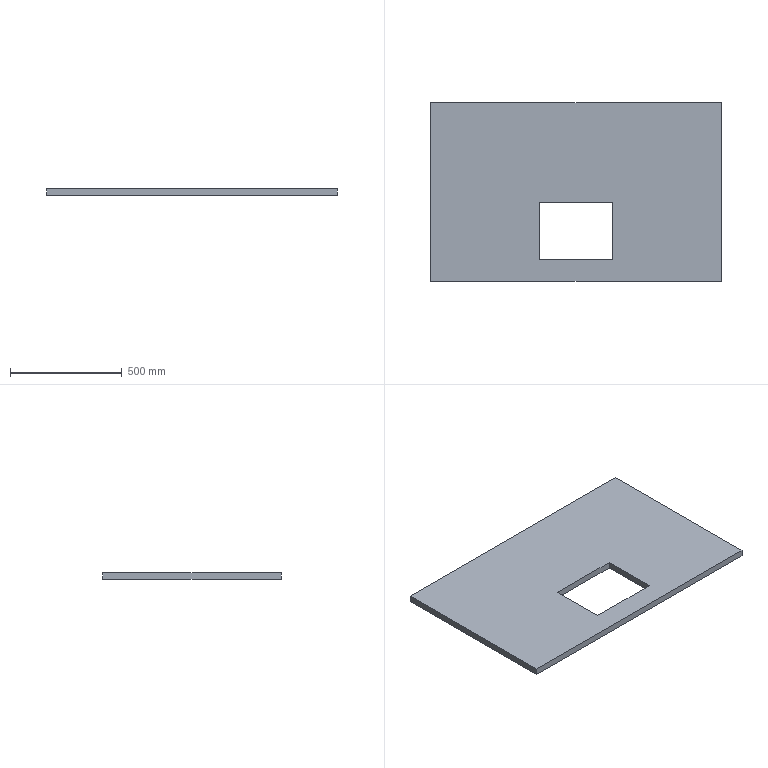Part | STEP file | Tube necking machine_id670_x_t | 1 solid | 10 faces | box 1300 x 800 x 30 mm | volume 28708260 mm3 | plane 10
STEP:
#1=CARTESIAN_POINT('',(0.,0.,0.));
#2=DIRECTION('',(0.,0.,1.));
#3=DIRECTION('',(1.,0.,0.));
#4=AXIS2_PLACEMENT_3D('',#1,#2,#3);
#5=CARTESIAN_POINT('',(-650.,400.,-30.));
#6=VERTEX_POINT('',#5);
#7=CARTESIAN_POINT('',(-650.,-400.,-30.));
#8=VERTEX_POINT('',#7);
#9=CARTESIAN_POINT('',(-650.,400.,-30.));
#10=DIRECTION('',(0.,-1.,0.));
#11=VECTOR('',#10,1.);
#12=LINE('',#9,#11);
#13=CARTESIAN_POINT('',(0.,0.,-30.));
#14=DIRECTION('',(0.,0.,1.));
#15=DIRECTION('',(1.,0.,0.));
#16=AXIS2_PLACEMENT_3D('',#13,#14,#15);
#17=PLANE('',#16);
#18=CARTESIAN_POINT('',(-650.,400.));
#19=DIRECTION('',(0.,-1.));
#20=VECTOR('',#19,1.);
#21=LINE('',#18,#20);
#22=(GEOMETRIC_REPRESENTATION_CONTEXT(2)PARAMETRIC_REPRESENTATION_CONTEXT()REPRESENTATION_CONTEXT('',''));
#23=DEFINITIONAL_REPRESENTATION('',(#21),#22);
#24=PCURVE('',#17,#23);
#25=CARTESIAN_POINT('',(-650.,400.,-30.));
#26=DIRECTION('',(-1.,0.,0.));
#27=DIRECTION('',(0.,0.,1.));
#28=AXIS2_PLACEMENT_3D('',#25,#26,#27);
#29=PLANE('',#28);
#30=CARTESIAN_POINT('',(0.,0.));
#31=DIRECTION('',(0.,-1.));
#32=VECTOR('',#31,1.);
#33=LINE('',#30,#32);
#34=(GEOMETRIC_REPRESENTATION_CONTEXT(2)PARAMETRIC_REPRESENTATION_CONTEXT()REPRESENTATION_CONTEXT('',''));
#35=DEFINITIONAL_REPRESENTATION('',(#33),#34);
#36=PCURVE('',#29,#35);
#37=SURFACE_CURVE('',#12,(#24,#36),.PCURVE_S1.);
#38=EDGE_CURVE('',#6,#8,#37,.T.);
#39=ORIENTED_EDGE('',*,*,#38,.F.);
#40=CARTESIAN_POINT('',(650.,400.,-30.));
#41=VERTEX_POINT('',#40);
#42=CARTESIAN_POINT('',(650.,400.,-30.));
#43=DIRECTION('',(-1.,0.,0.));
#44=VECTOR('',#43,1.);
#45=LINE('',#42,#44);
#46=CARTESIAN_POINT('',(650.,400.));
#47=DIRECTION('',(-1.,0.));
#48=VECTOR('',#47,1.);
#49=LINE('',#46,#48);
#50=(GEOMETRIC_REPRESENTATION_CONTEXT(2)PARAMETRIC_REPRESENTATION_CONTEXT()REPRESENTATION_CONTEXT('',''));
#51=DEFINITIONAL_REPRESENTATION('',(#49),#50);
#52=PCURVE('',#17,#51);
#53=CARTESIAN_POINT('',(650.,400.,-30.));
#54=DIRECTION('',(0.,1.,0.));
#55=DIRECTION('',(0.,0.,1.));
#56=AXIS2_PLACEMENT_3D('',#53,#54,#55);
#57=PLANE('',#56);
#58=CARTESIAN_POINT('',(0.,0.));
#59=DIRECTION('',(0.,-1.));
#60=VECTOR('',#59,1.);
#61=LINE('',#58,#60);
#62=(GEOMETRIC_REPRESENTATION_CONTEXT(2)PARAMETRIC_REPRESENTATION_CONTEXT()REPRESENTATION_CONTEXT('',''));
#63=DEFINITIONAL_REPRESENTATION('',(#61),#62);
#64=PCURVE('',#57,#63);
#65=SURFACE_CURVE('',#45,(#52,#64),.PCURVE_S1.);
#66=EDGE_CURVE('',#41,#6,#65,.T.);
#67=ORIENTED_EDGE('',*,*,#66,.F.);
#68=CARTESIAN_POINT('',(650.,-400.,-30.));
#69=VERTEX_POINT('',#68);
#70=CARTESIAN_POINT('',(650.,-400.,-30.));
#71=DIRECTION('',(0.,1.,0.));
#72=VECTOR('',#71,1.);
#73=LINE('',#70,#72);
#74=CARTESIAN_POINT('',(650.,-400.));
#75=DIRECTION('',(0.,1.));
#76=VECTOR('',#75,1.);
#77=LINE('',#74,#76);
#78=(GEOMETRIC_REPRESENTATION_CONTEXT(2)PARAMETRIC_REPRESENTATION_CONTEXT()REPRESENTATION_CONTEXT('',''));
#79=DEFINITIONAL_REPRESENTATION('',(#77),#78);
#80=PCURVE('',#17,#79);
#81=CARTESIAN_POINT('',(650.,-400.,-30.));
#82=DIRECTION('',(1.,0.,0.));
#83=DIRECTION('',(0.,0.,-1.));
#84=AXIS2_PLACEMENT_3D('',#81,#82,#83);
#85=PLANE('',#84);
#86=CARTESIAN_POINT('',(0.,0.));
#87=DIRECTION('',(0.,1.));
#88=VECTOR('',#87,1.);
#89=LINE('',#86,#88);
#90=(GEOMETRIC_REPRESENTATION_CONTEXT(2)PARAMETRIC_REPRESENTATION_CONTEXT()REPRESENTATION_CONTEXT('',''));
#91=DEFINITIONAL_REPRESENTATION('',(#89),#90);
#92=PCURVE('',#85,#91);
#93=SURFACE_CURVE('',#73,(#80,#92),.PCURVE_S1.);
#94=EDGE_CURVE('',#69,#41,#93,.T.);
#95=ORIENTED_EDGE('',*,*,#94,.F.);
#96=CARTESIAN_POINT('',(-650.,-400.,-30.));
#97=DIRECTION('',(1.,0.,0.));
#98=VECTOR('',#97,1.);
#99=LINE('',#96,#98);
#100=CARTESIAN_POINT('',(-650.,-400.));
#101=DIRECTION('',(1.,0.));
#102=VECTOR('',#101,1.);
#103=LINE('',#100,#102);
#104=(GEOMETRIC_REPRESENTATION_CONTEXT(2)PARAMETRIC_REPRESENTATION_CONTEXT()REPRESENTATION_CONTEXT('',''));
#105=DEFINITIONAL_REPRESENTATION('',(#103),#104);
#106=PCURVE('',#17,#105);
#107=CARTESIAN_POINT('',(-650.,-400.,-30.));
#108=DIRECTION('',(0.,-1.,0.));
#109=DIRECTION('',(0.,0.,-1.));
#110=AXIS2_PLACEMENT_3D('',#107,#108,#109);
#111=PLANE('',#110);
#112=CARTESIAN_POINT('',(0.,0.));
#113=DIRECTION('',(0.,1.));
#114=VECTOR('',#113,1.);
#115=LINE('',#112,#114);
#116=(GEOMETRIC_REPRESENTATION_CONTEXT(2)PARAMETRIC_REPRESENTATION_CONTEXT()REPRESENTATION_CONTEXT('',''));
#117=DEFINITIONAL_REPRESENTATION('',(#115),#116);
#118=PCURVE('',#111,#117);
#119=SURFACE_CURVE('',#99,(#106,#118),.PCURVE_S1.);
#120=EDGE_CURVE('',#8,#69,#119,.T.);
#121=ORIENTED_EDGE('',*,*,#120,.F.);
#122=EDGE_LOOP('',(#39,#67,#95,#121));
#123=FACE_BOUND('',#122,.T.);
#124=CARTESIAN_POINT('',(-163.5,-46.,-30.));
#125=VERTEX_POINT('',#124);
#126=CARTESIAN_POINT('',(-163.5,-300.,-30.));
#127=VERTEX_POINT('',#126);
#128=CARTESIAN_POINT('',(-163.5,0.,-30.));
#129=DIRECTION('',(0.,-1.,0.));
#130=VECTOR('',#129,1.);
#131=LINE('',#128,#130);
#132=CARTESIAN_POINT('',(-163.5,0.));
#133=DIRECTION('',(0.,-1.));
#134=VECTOR('',#133,1.);
#135=LINE('',#132,#134);
#136=(GEOMETRIC_REPRESENTATION_CONTEXT(2)PARAMETRIC_REPRESENTATION_CONTEXT()REPRESENTATION_CONTEXT('',''));
#137=DEFINITIONAL_REPRESENTATION('',(#135),#136);
#138=PCURVE('',#17,#137);
#139=CARTESIAN_POINT('',(-163.5,-46.,30.));
#140=DIRECTION('',(1.,0.,0.));
#141=DIRECTION('',(0.,0.,-1.));
#142=AXIS2_PLACEMENT_3D('',#139,#140,#141);
#143=PLANE('',#142);
#144=CARTESIAN_POINT('',(60.,46.));
#145=DIRECTION('',(0.,-1.));
#146=VECTOR('',#145,1.);
#147=LINE('',#144,#146);
#148=(GEOMETRIC_REPRESENTATION_CONTEXT(2)PARAMETRIC_REPRESENTATION_CONTEXT()REPRESENTATION_CONTEXT('',''));
#149=DEFINITIONAL_REPRESENTATION('',(#147),#148);
#150=PCURVE('',#143,#149);
#151=SURFACE_CURVE('',#131,(#138,#150),.PCURVE_S1.);
#152=EDGE_CURVE('',#125,#127,#151,.T.);
#153=ORIENTED_EDGE('',*,*,#152,.T.);
#154=CARTESIAN_POINT('',(163.5,-300.,-30.));
#155=VERTEX_POINT('',#154);
#156=CARTESIAN_POINT('',(0.,-300.,-30.));
#157=DIRECTION('',(1.,0.,0.));
#158=VECTOR('',#157,1.);
#159=LINE('',#156,#158);
#160=CARTESIAN_POINT('',(0.,-300.));
#161=DIRECTION('',(1.,0.));
#162=VECTOR('',#161,1.);
#163=LINE('',#160,#162);
#164=(GEOMETRIC_REPRESENTATION_CONTEXT(2)PARAMETRIC_REPRESENTATION_CONTEXT()REPRESENTATION_CONTEXT('',''));
#165=DEFINITIONAL_REPRESENTATION('',(#163),#164);
#166=PCURVE('',#17,#165);
#167=CARTESIAN_POINT('',(-163.5,-300.,30.));
#168=DIRECTION('',(0.,1.,0.));
#169=DIRECTION('',(0.,0.,1.));
#170=AXIS2_PLACEMENT_3D('',#167,#168,#169);
#171=PLANE('',#170);
#172=CARTESIAN_POINT('',(-60.,163.5));
#173=DIRECTION('',(0.,1.));
#174=VECTOR('',#173,1.);
#175=LINE('',#172,#174);
#176=(GEOMETRIC_REPRESENTATION_CONTEXT(2)PARAMETRIC_REPRESENTATION_CONTEXT()REPRESENTATION_CONTEXT('',''));
#177=DEFINITIONAL_REPRESENTATION('',(#175),#176);
#178=PCURVE('',#171,#177);
#179=SURFACE_CURVE('',#159,(#166,#178),.PCURVE_S1.);
#180=EDGE_CURVE('',#127,#155,#179,.T.);
#181=ORIENTED_EDGE('',*,*,#180,.T.);
#182=CARTESIAN_POINT('',(163.5,-46.,-30.));
#183=VERTEX_POINT('',#182);
#184=CARTESIAN_POINT('',(163.5,0.,-30.));
#185=DIRECTION('',(0.,1.,0.));
#186=VECTOR('',#185,1.);
#187=LINE('',#184,#186);
#188=CARTESIAN_POINT('',(163.5,0.));
#189=DIRECTION('',(0.,1.));
#190=VECTOR('',#189,1.);
#191=LINE('',#188,#190);
#192=(GEOMETRIC_REPRESENTATION_CONTEXT(2)PARAMETRIC_REPRESENTATION_CONTEXT()REPRESENTATION_CONTEXT('',''));
#193=DEFINITIONAL_REPRESENTATION('',(#191),#192);
#194=PCURVE('',#17,#193);
#195=CARTESIAN_POINT('',(163.5,-300.,30.));
#196=DIRECTION('',(-1.,0.,0.));
#197=DIRECTION('',(0.,-1.,0.));
#198=AXIS2_PLACEMENT_3D('',#195,#196,#197);
#199=PLANE('',#198);
#200=CARTESIAN_POINT('',(-300.,-60.));
#201=DIRECTION('',(-1.,0.));
#202=VECTOR('',#201,1.);
#203=LINE('',#200,#202);
#204=(GEOMETRIC_REPRESENTATION_CONTEXT(2)PARAMETRIC_REPRESENTATION_CONTEXT()REPRESENTATION_CONTEXT('',''));
#205=DEFINITIONAL_REPRESENTATION('',(#203),#204);
#206=PCURVE('',#199,#205);
#207=SURFACE_CURVE('',#187,(#194,#206),.PCURVE_S1.);
#208=EDGE_CURVE('',#155,#183,#207,.T.);
#209=ORIENTED_EDGE('',*,*,#208,.T.);
#210=CARTESIAN_POINT('',(0.,-46.,-30.));
#211=DIRECTION('',(-1.,0.,0.));
#212=VECTOR('',#211,1.);
#213=LINE('',#210,#212);
#214=CARTESIAN_POINT('',(0.,-46.));
#215=DIRECTION('',(-1.,0.));
#216=VECTOR('',#215,1.);
#217=LINE('',#214,#216);
#218=(GEOMETRIC_REPRESENTATION_CONTEXT(2)PARAMETRIC_REPRESENTATION_CONTEXT()REPRESENTATION_CONTEXT('',''));
#219=DEFINITIONAL_REPRESENTATION('',(#217),#218);
#220=PCURVE('',#17,#219);
#221=CARTESIAN_POINT('',(163.5,-46.,30.));
#222=DIRECTION('',(0.,-1.,0.));
#223=DIRECTION('',(0.,0.,-1.));
#224=AXIS2_PLACEMENT_3D('',#221,#222,#223);
#225=PLANE('',#224);
#226=CARTESIAN_POINT('',(60.,-163.5));
#227=DIRECTION('',(0.,-1.));
#228=VECTOR('',#227,1.);
#229=LINE('',#226,#228);
#230=(GEOMETRIC_REPRESENTATION_CONTEXT(2)PARAMETRIC_REPRESENTATION_CONTEXT()REPRESENTATION_CONTEXT('',''));
#231=DEFINITIONAL_REPRESENTATION('',(#229),#230);
#232=PCURVE('',#225,#231);
#233=SURFACE_CURVE('',#213,(#220,#232),.PCURVE_S1.);
#234=EDGE_CURVE('',#183,#125,#233,.T.);
#235=ORIENTED_EDGE('',*,*,#234,.T.);
#236=EDGE_LOOP('',(#153,#181,#209,#235));
#237=FACE_BOUND('',#236,.T.);
#238=ADVANCED_FACE('',(#123,#237),#17,.F.);
#239=CARTESIAN_POINT('',(-650.,400.,0.));
#240=VERTEX_POINT('',#239);
#241=CARTESIAN_POINT('',(-650.,-400.,0.));
#242=VERTEX_POINT('',#241);
#243=CARTESIAN_POINT('',(-650.,400.,0.));
#244=DIRECTION('',(0.,-1.,0.));
#245=VECTOR('',#244,1.);
#246=LINE('',#243,#245);
#247=CARTESIAN_POINT('',(0.,0.,0.));
#248=DIRECTION('',(0.,0.,1.));
#249=DIRECTION('',(1.,0.,0.));
#250=AXIS2_PLACEMENT_3D('',#247,#248,#249);
#251=PLANE('',#250);
#252=CARTESIAN_POINT('',(-650.,400.));
#253=DIRECTION('',(0.,-1.));
#254=VECTOR('',#253,1.);
#255=LINE('',#252,#254);
#256=(GEOMETRIC_REPRESENTATION_CONTEXT(2)PARAMETRIC_REPRESENTATION_CONTEXT()REPRESENTATION_CONTEXT('',''));
#257=DEFINITIONAL_REPRESENTATION('',(#255),#256);
#258=PCURVE('',#251,#257);
#259=CARTESIAN_POINT('',(30.,0.));
#260=DIRECTION('',(0.,-1.));
#261=VECTOR('',#260,1.);
#262=LINE('',#259,#261);
#263=(GEOMETRIC_REPRESENTATION_CONTEXT(2)PARAMETRIC_REPRESENTATION_CONTEXT()REPRESENTATION_CONTEXT('',''));
#264=DEFINITIONAL_REPRESENTATION('',(#262),#263);
#265=PCURVE('',#29,#264);
#266=SURFACE_CURVE('',#246,(#258,#265),.PCURVE_S1.);
#267=EDGE_CURVE('',#240,#242,#266,.T.);
#268=ORIENTED_EDGE('',*,*,#267,.T.);
#269=CARTESIAN_POINT('',(650.,-400.,0.));
#270=VERTEX_POINT('',#269);
#271=CARTESIAN_POINT('',(-650.,-400.,0.));
#272=DIRECTION('',(1.,0.,0.));
#273=VECTOR('',#272,1.);
#274=LINE('',#271,#273);
#275=CARTESIAN_POINT('',(-650.,-400.));
#276=DIRECTION('',(1.,0.));
#277=VECTOR('',#276,1.);
#278=LINE('',#275,#277);
#279=(GEOMETRIC_REPRESENTATION_CONTEXT(2)PARAMETRIC_REPRESENTATION_CONTEXT()REPRESENTATION_CONTEXT('',''));
#280=DEFINITIONAL_REPRESENTATION('',(#278),#279);
#281=PCURVE('',#251,#280);
#282=CARTESIAN_POINT('',(-30.,0.));
#283=DIRECTION('',(0.,1.));
#284=VECTOR('',#283,1.);
#285=LINE('',#282,#284);
#286=(GEOMETRIC_REPRESENTATION_CONTEXT(2)PARAMETRIC_REPRESENTATION_CONTEXT()REPRESENTATION_CONTEXT('',''));
#287=DEFINITIONAL_REPRESENTATION('',(#285),#286);
#288=PCURVE('',#111,#287);
#289=SURFACE_CURVE('',#274,(#281,#288),.PCURVE_S1.);
#290=EDGE_CURVE('',#242,#270,#289,.T.);
#291=ORIENTED_EDGE('',*,*,#290,.T.);
#292=CARTESIAN_POINT('',(650.,400.,0.));
#293=VERTEX_POINT('',#292);
#294=CARTESIAN_POINT('',(650.,-400.,0.));
#295=DIRECTION('',(0.,1.,0.));
#296=VECTOR('',#295,1.);
#297=LINE('',#294,#296);
#298=CARTESIAN_POINT('',(650.,-400.));
#299=DIRECTION('',(0.,1.));
#300=VECTOR('',#299,1.);
#301=LINE('',#298,#300);
#302=(GEOMETRIC_REPRESENTATION_CONTEXT(2)PARAMETRIC_REPRESENTATION_CONTEXT()REPRESENTATION_CONTEXT('',''));
#303=DEFINITIONAL_REPRESENTATION('',(#301),#302);
#304=PCURVE('',#251,#303);
#305=CARTESIAN_POINT('',(-30.,0.));
#306=DIRECTION('',(0.,1.));
#307=VECTOR('',#306,1.);
#308=LINE('',#305,#307);
#309=(GEOMETRIC_REPRESENTATION_CONTEXT(2)PARAMETRIC_REPRESENTATION_CONTEXT()REPRESENTATION_CONTEXT('',''));
#310=DEFINITIONAL_REPRESENTATION('',(#308),#309);
#311=PCURVE('',#85,#310);
#312=SURFACE_CURVE('',#297,(#304,#311),.PCURVE_S1.);
#313=EDGE_CURVE('',#270,#293,#312,.T.);
#314=ORIENTED_EDGE('',*,*,#313,.T.);
#315=CARTESIAN_POINT('',(650.,400.,0.));
#316=DIRECTION('',(-1.,0.,0.));
#317=VECTOR('',#316,1.);
#318=LINE('',#315,#317);
#319=CARTESIAN_POINT('',(650.,400.));
#320=DIRECTION('',(-1.,0.));
#321=VECTOR('',#320,1.);
#322=LINE('',#319,#321);
#323=(GEOMETRIC_REPRESENTATION_CONTEXT(2)PARAMETRIC_REPRESENTATION_CONTEXT()REPRESENTATION_CONTEXT('',''));
#324=DEFINITIONAL_REPRESENTATION('',(#322),#323);
#325=PCURVE('',#251,#324);
#326=CARTESIAN_POINT('',(30.,0.));
#327=DIRECTION('',(0.,-1.));
#328=VECTOR('',#327,1.);
#329=LINE('',#326,#328);
#330=(GEOMETRIC_REPRESENTATION_CONTEXT(2)PARAMETRIC_REPRESENTATION_CONTEXT()REPRESENTATION_CONTEXT('',''));
#331=DEFINITIONAL_REPRESENTATION('',(#329),#330);
#332=PCURVE('',#57,#331);
#333=SURFACE_CURVE('',#318,(#325,#332),.PCURVE_S1.);
#334=EDGE_CURVE('',#293,#240,#333,.T.);
#335=ORIENTED_EDGE('',*,*,#334,.T.);
#336=EDGE_LOOP('',(#268,#291,#314,#335));
#337=FACE_BOUND('',#336,.T.);
#338=CARTESIAN_POINT('',(-163.5,-300.,0.));
#339=VERTEX_POINT('',#338);
#340=CARTESIAN_POINT('',(163.5,-300.,0.));
#341=VERTEX_POINT('',#340);
#342=CARTESIAN_POINT('',(0.,-300.,0.));
#343=DIRECTION('',(1.,0.,0.));
#344=VECTOR('',#343,1.);
#345=LINE('',#342,#344);
#346=CARTESIAN_POINT('',(0.,-300.));
#347=DIRECTION('',(1.,0.));
#348=VECTOR('',#347,1.);
#349=LINE('',#346,#348);
#350=(GEOMETRIC_REPRESENTATION_CONTEXT(2)PARAMETRIC_REPRESENTATION_CONTEXT()REPRESENTATION_CONTEXT('',''));
#351=DEFINITIONAL_REPRESENTATION('',(#349),#350);
#352=PCURVE('',#251,#351);
#353=CARTESIAN_POINT('',(-30.,163.5));
#354=DIRECTION('',(0.,1.));
#355=VECTOR('',#354,1.);
#356=LINE('',#353,#355);
#357=(GEOMETRIC_REPRESENTATION_CONTEXT(2)PARAMETRIC_REPRESENTATION_CONTEXT()REPRESENTATION_CONTEXT('',''));
#358=DEFINITIONAL_REPRESENTATION('',(#356),#357);
#359=PCURVE('',#171,#358);
#360=SURFACE_CURVE('',#345,(#352,#359),.PCURVE_S1.);
#361=EDGE_CURVE('',#339,#341,#360,.T.);
#362=ORIENTED_EDGE('',*,*,#361,.F.);
#363=CARTESIAN_POINT('',(-163.5,-46.,0.));
#364=VERTEX_POINT('',#363);
#365=CARTESIAN_POINT('',(-163.5,0.,0.));
#366=DIRECTION('',(0.,-1.,0.));
#367=VECTOR('',#366,1.);
#368=LINE('',#365,#367);
#369=CARTESIAN_POINT('',(-163.5,0.));
#370=DIRECTION('',(0.,-1.));
#371=VECTOR('',#370,1.);
#372=LINE('',#369,#371);
#373=(GEOMETRIC_REPRESENTATION_CONTEXT(2)PARAMETRIC_REPRESENTATION_CONTEXT()REPRESENTATION_CONTEXT('',''));
#374=DEFINITIONAL_REPRESENTATION('',(#372),#373);
#375=PCURVE('',#251,#374);
#376=CARTESIAN_POINT('',(30.,46.));
#377=DIRECTION('',(0.,-1.));
#378=VECTOR('',#377,1.);
#379=LINE('',#376,#378);
#380=(GEOMETRIC_REPRESENTATION_CONTEXT(2)PARAMETRIC_REPRESENTATION_CONTEXT()REPRESENTATION_CONTEXT('',''));
#381=DEFINITIONAL_REPRESENTATION('',(#379),#380);
#382=PCURVE('',#143,#381);
#383=SURFACE_CURVE('',#368,(#375,#382),.PCURVE_S1.);
#384=EDGE_CURVE('',#364,#339,#383,.T.);
#385=ORIENTED_EDGE('',*,*,#384,.F.);
#386=CARTESIAN_POINT('',(163.5,-46.,0.));
#387=VERTEX_POINT('',#386);
#388=CARTESIAN_POINT('',(0.,-46.,0.));
#389=DIRECTION('',(-1.,0.,0.));
#390=VECTOR('',#389,1.);
#391=LINE('',#388,#390);
#392=CARTESIAN_POINT('',(0.,-46.));
#393=DIRECTION('',(-1.,0.));
#394=VECTOR('',#393,1.);
#395=LINE('',#392,#394);
#396=(GEOMETRIC_REPRESENTATION_CONTEXT(2)PARAMETRIC_REPRESENTATION_CONTEXT()REPRESENTATION_CONTEXT('',''));
#397=DEFINITIONAL_REPRESENTATION('',(#395),#396);
#398=PCURVE('',#251,#397);
#399=CARTESIAN_POINT('',(30.,-163.5));
#400=DIRECTION('',(0.,-1.));
#401=VECTOR('',#400,1.);
#402=LINE('',#399,#401);
#403=(GEOMETRIC_REPRESENTATION_CONTEXT(2)PARAMETRIC_REPRESENTATION_CONTEXT()REPRESENTATION_CONTEXT('',''));
#404=DEFINITIONAL_REPRESENTATION('',(#402),#403);
#405=PCURVE('',#225,#404);
#406=SURFACE_CURVE('',#391,(#398,#405),.PCURVE_S1.);
#407=EDGE_CURVE('',#387,#364,#406,.T.);
#408=ORIENTED_EDGE('',*,*,#407,.F.);
#409=CARTESIAN_POINT('',(163.5,0.,0.));
#410=DIRECTION('',(0.,1.,0.));
#411=VECTOR('',#410,1.);
#412=LINE('',#409,#411);
#413=CARTESIAN_POINT('',(163.5,0.));
#414=DIRECTION('',(0.,1.));
#415=VECTOR('',#414,1.);
#416=LINE('',#413,#415);
#417=(GEOMETRIC_REPRESENTATION_CONTEXT(2)PARAMETRIC_REPRESENTATION_CONTEXT()REPRESENTATION_CONTEXT('',''));
#418=DEFINITIONAL_REPRESENTATION('',(#416),#417);
#419=PCURVE('',#251,#418);
#420=CARTESIAN_POINT('',(-300.,-30.));
#421=DIRECTION('',(-1.,0.));
#422=VECTOR('',#421,1.);
#423=LINE('',#420,#422);
#424=(GEOMETRIC_REPRESENTATION_CONTEXT(2)PARAMETRIC_REPRESENTATION_CONTEXT()REPRESENTATION_CONTEXT('',''));
#425=DEFINITIONAL_REPRESENTATION('',(#423),#424);
#426=PCURVE('',#199,#425);
#427=SURFACE_CURVE('',#412,(#419,#426),.PCURVE_S1.);
#428=EDGE_CURVE('',#341,#387,#427,.T.);
#429=ORIENTED_EDGE('',*,*,#428,.F.);
#430=EDGE_LOOP('',(#362,#385,#408,#429));
#431=FACE_BOUND('',#430,.T.);
#432=ADVANCED_FACE('',(#337,#431),#251,.T.);
#433=ORIENTED_EDGE('',*,*,#267,.F.);
#434=CARTESIAN_POINT('',(-650.,400.,-30.));
#435=DIRECTION('',(0.,0.,1.));
#436=VECTOR('',#435,1.);
#437=LINE('',#434,#436);
#438=CARTESIAN_POINT('',(0.,0.));
#439=DIRECTION('',(1.,0.));
#440=VECTOR('',#439,1.);
#441=LINE('',#438,#440);
#442=(GEOMETRIC_REPRESENTATION_CONTEXT(2)PARAMETRIC_REPRESENTATION_CONTEXT()REPRESENTATION_CONTEXT('',''));
#443=DEFINITIONAL_REPRESENTATION('',(#441),#442);
#444=PCURVE('',#29,#443);
#445=CARTESIAN_POINT('',(0.,-1300.));
#446=DIRECTION('',(1.,0.));
#447=VECTOR('',#446,1.);
#448=LINE('',#445,#447);
#449=(GEOMETRIC_REPRESENTATION_CONTEXT(2)PARAMETRIC_REPRESENTATION_CONTEXT()REPRESENTATION_CONTEXT('',''));
#450=DEFINITIONAL_REPRESENTATION('',(#448),#449);
#451=PCURVE('',#57,#450);
#452=SURFACE_CURVE('',#437,(#444,#451),.PCURVE_S1.);
#453=EDGE_CURVE('',#6,#240,#452,.T.);
#454=ORIENTED_EDGE('',*,*,#453,.F.);
#455=ORIENTED_EDGE('',*,*,#38,.T.);
#456=CARTESIAN_POINT('',(-650.,-400.,-30.));
#457=DIRECTION('',(0.,0.,1.));
#458=VECTOR('',#457,1.);
#459=LINE('',#456,#458);
#460=CARTESIAN_POINT('',(0.,-800.));
#461=DIRECTION('',(1.,0.));
#462=VECTOR('',#461,1.);
#463=LINE('',#460,#462);
#464=(GEOMETRIC_REPRESENTATION_CONTEXT(2)PARAMETRIC_REPRESENTATION_CONTEXT()REPRESENTATION_CONTEXT('',''));
#465=DEFINITIONAL_REPRESENTATION('',(#463),#464);
#466=PCURVE('',#29,#465);
#467=CARTESIAN_POINT('',(0.,0.));
#468=DIRECTION('',(-1.,0.));
#469=VECTOR('',#468,1.);
#470=LINE('',#467,#469);
#471=(GEOMETRIC_REPRESENTATION_CONTEXT(2)PARAMETRIC_REPRESENTATION_CONTEXT()REPRESENTATION_CONTEXT('',''));
#472=DEFINITIONAL_REPRESENTATION('',(#470),#471);
#473=PCURVE('',#111,#472);
#474=SURFACE_CURVE('',#459,(#466,#473),.PCURVE_S1.);
#475=EDGE_CURVE('',#8,#242,#474,.T.);
#476=ORIENTED_EDGE('',*,*,#475,.T.);
#477=EDGE_LOOP('',(#433,#454,#455,#476));
#478=FACE_BOUND('',#477,.T.);
#479=ADVANCED_FACE('',(#478),#29,.T.);
#480=ORIENTED_EDGE('',*,*,#290,.F.);
#481=ORIENTED_EDGE('',*,*,#475,.F.);
#482=ORIENTED_EDGE('',*,*,#120,.T.);
#483=CARTESIAN_POINT('',(650.,-400.,-30.));
#484=DIRECTION('',(0.,0.,1.));
#485=VECTOR('',#484,1.);
#486=LINE('',#483,#485);
#487=CARTESIAN_POINT('',(0.,1300.));
#488=DIRECTION('',(-1.,0.));
#489=VECTOR('',#488,1.);
#490=LINE('',#487,#489);
#491=(GEOMETRIC_REPRESENTATION_CONTEXT(2)PARAMETRIC_REPRESENTATION_CONTEXT()REPRESENTATION_CONTEXT('',''));
#492=DEFINITIONAL_REPRESENTATION('',(#490),#491);
#493=PCURVE('',#111,#492);
#494=CARTESIAN_POINT('',(0.,0.));
#495=DIRECTION('',(-1.,0.));
#496=VECTOR('',#495,1.);
#497=LINE('',#494,#496);
#498=(GEOMETRIC_REPRESENTATION_CONTEXT(2)PARAMETRIC_REPRESENTATION_CONTEXT()REPRESENTATION_CONTEXT('',''));
#499=DEFINITIONAL_REPRESENTATION('',(#497),#498);
#500=PCURVE('',#85,#499);
#501=SURFACE_CURVE('',#486,(#493,#500),.PCURVE_S1.);
#502=EDGE_CURVE('',#69,#270,#501,.T.);
#503=ORIENTED_EDGE('',*,*,#502,.T.);
#504=EDGE_LOOP('',(#480,#481,#482,#503));
#505=FACE_BOUND('',#504,.T.);
#506=ADVANCED_FACE('',(#505),#111,.T.);
#507=ORIENTED_EDGE('',*,*,#313,.F.);
#508=ORIENTED_EDGE('',*,*,#502,.F.);
#509=ORIENTED_EDGE('',*,*,#94,.T.);
#510=CARTESIAN_POINT('',(650.,400.,-30.));
#511=DIRECTION('',(0.,0.,1.));
#512=VECTOR('',#511,1.);
#513=LINE('',#510,#512);
#514=CARTESIAN_POINT('',(0.,800.));
#515=DIRECTION('',(-1.,0.));
#516=VECTOR('',#515,1.);
#517=LINE('',#514,#516);
#518=(GEOMETRIC_REPRESENTATION_CONTEXT(2)PARAMETRIC_REPRESENTATION_CONTEXT()REPRESENTATION_CONTEXT('',''));
#519=DEFINITIONAL_REPRESENTATION('',(#517),#518);
#520=PCURVE('',#85,#519);
#521=CARTESIAN_POINT('',(0.,0.));
#522=DIRECTION('',(1.,0.));
#523=VECTOR('',#522,1.);
#524=LINE('',#521,#523);
#525=(GEOMETRIC_REPRESENTATION_CONTEXT(2)PARAMETRIC_REPRESENTATION_CONTEXT()REPRESENTATION_CONTEXT('',''));
#526=DEFINITIONAL_REPRESENTATION('',(#524),#525);
#527=PCURVE('',#57,#526);
#528=SURFACE_CURVE('',#513,(#520,#527),.PCURVE_S1.);
#529=EDGE_CURVE('',#41,#293,#528,.T.);
#530=ORIENTED_EDGE('',*,*,#529,.T.);
#531=EDGE_LOOP('',(#507,#508,#509,#530));
#532=FACE_BOUND('',#531,.T.);
#533=ADVANCED_FACE('',(#532),#85,.T.);
#534=ORIENTED_EDGE('',*,*,#334,.F.);
#535=ORIENTED_EDGE('',*,*,#529,.F.);
#536=ORIENTED_EDGE('',*,*,#66,.T.);
#537=ORIENTED_EDGE('',*,*,#453,.T.);
#538=EDGE_LOOP('',(#534,#535,#536,#537));
#539=FACE_BOUND('',#538,.T.);
#540=ADVANCED_FACE('',(#539),#57,.T.);
#541=ORIENTED_EDGE('',*,*,#152,.F.);
#542=CARTESIAN_POINT('',(-163.5,-46.,30.));
#543=DIRECTION('',(0.,0.,1.));
#544=VECTOR('',#543,1.);
#545=LINE('',#542,#544);
#546=CARTESIAN_POINT('',(0.,0.));
#547=DIRECTION('',(-1.,0.));
#548=VECTOR('',#547,1.);
#549=LINE('',#546,#548);
#550=(GEOMETRIC_REPRESENTATION_CONTEXT(2)PARAMETRIC_REPRESENTATION_CONTEXT()REPRESENTATION_CONTEXT('',''));
#551=DEFINITIONAL_REPRESENTATION('',(#549),#550);
#552=PCURVE('',#143,#551);
#553=CARTESIAN_POINT('',(0.,-327.));
#554=DIRECTION('',(-1.,0.));
#555=VECTOR('',#554,1.);
#556=LINE('',#553,#555);
#557=(GEOMETRIC_REPRESENTATION_CONTEXT(2)PARAMETRIC_REPRESENTATION_CONTEXT()REPRESENTATION_CONTEXT('',''));
#558=DEFINITIONAL_REPRESENTATION('',(#556),#557);
#559=PCURVE('',#225,#558);
#560=SURFACE_CURVE('',#545,(#552,#559),.PCURVE_S1.);
#561=EDGE_CURVE('',#125,#364,#560,.T.);
#562=ORIENTED_EDGE('',*,*,#561,.T.);
#563=ORIENTED_EDGE('',*,*,#384,.T.);
#564=CARTESIAN_POINT('',(-163.5,-300.,30.));
#565=DIRECTION('',(0.,0.,1.));
#566=VECTOR('',#565,1.);
#567=LINE('',#564,#566);
#568=CARTESIAN_POINT('',(0.,-254.));
#569=DIRECTION('',(-1.,0.));
#570=VECTOR('',#569,1.);
#571=LINE('',#568,#570);
#572=(GEOMETRIC_REPRESENTATION_CONTEXT(2)PARAMETRIC_REPRESENTATION_CONTEXT()REPRESENTATION_CONTEXT('',''));
#573=DEFINITIONAL_REPRESENTATION('',(#571),#572);
#574=PCURVE('',#143,#573);
#575=CARTESIAN_POINT('',(0.,0.));
#576=DIRECTION('',(1.,0.));
#577=VECTOR('',#576,1.);
#578=LINE('',#575,#577);
#579=(GEOMETRIC_REPRESENTATION_CONTEXT(2)PARAMETRIC_REPRESENTATION_CONTEXT()REPRESENTATION_CONTEXT('',''));
#580=DEFINITIONAL_REPRESENTATION('',(#578),#579);
#581=PCURVE('',#171,#580);
#582=SURFACE_CURVE('',#567,(#574,#581),.PCURVE_S1.);
#583=EDGE_CURVE('',#127,#339,#582,.T.);
#584=ORIENTED_EDGE('',*,*,#583,.F.);
#585=EDGE_LOOP('',(#541,#562,#563,#584));
#586=FACE_BOUND('',#585,.T.);
#587=ADVANCED_FACE('',(#586),#143,.T.);
#588=ORIENTED_EDGE('',*,*,#180,.F.);
#589=ORIENTED_EDGE('',*,*,#583,.T.);
#590=ORIENTED_EDGE('',*,*,#361,.T.);
#591=CARTESIAN_POINT('',(163.5,-300.,30.));
#592=DIRECTION('',(0.,0.,1.));
#593=VECTOR('',#592,1.);
#594=LINE('',#591,#593);
#595=CARTESIAN_POINT('',(0.,327.));
#596=DIRECTION('',(1.,0.));
#597=VECTOR('',#596,1.);
#598=LINE('',#595,#597);
#599=(GEOMETRIC_REPRESENTATION_CONTEXT(2)PARAMETRIC_REPRESENTATION_CONTEXT()REPRESENTATION_CONTEXT('',''));
#600=DEFINITIONAL_REPRESENTATION('',(#598),#599);
#601=PCURVE('',#171,#600);
#602=CARTESIAN_POINT('',(0.,0.));
#603=DIRECTION('',(0.,1.));
#604=VECTOR('',#603,1.);
#605=LINE('',#602,#604);
#606=(GEOMETRIC_REPRESENTATION_CONTEXT(2)PARAMETRIC_REPRESENTATION_CONTEXT()REPRESENTATION_CONTEXT('',''));
#607=DEFINITIONAL_REPRESENTATION('',(#605),#606);
#608=PCURVE('',#199,#607);
#609=SURFACE_CURVE('',#594,(#601,#608),.PCURVE_S1.);
#610=EDGE_CURVE('',#155,#341,#609,.T.);
#611=ORIENTED_EDGE('',*,*,#610,.F.);
#612=EDGE_LOOP('',(#588,#589,#590,#611));
#613=FACE_BOUND('',#612,.T.);
#614=ADVANCED_FACE('',(#613),#171,.T.);
#615=ORIENTED_EDGE('',*,*,#208,.F.);
#616=ORIENTED_EDGE('',*,*,#610,.T.);
#617=ORIENTED_EDGE('',*,*,#428,.T.);
#618=CARTESIAN_POINT('',(163.5,-46.,30.));
#619=DIRECTION('',(0.,0.,1.));
#620=VECTOR('',#619,1.);
#621=LINE('',#618,#620);
#622=CARTESIAN_POINT('',(-254.,0.));
#623=DIRECTION('',(0.,1.));
#624=VECTOR('',#623,1.);
#625=LINE('',#622,#624);
#626=(GEOMETRIC_REPRESENTATION_CONTEXT(2)PARAMETRIC_REPRESENTATION_CONTEXT()REPRESENTATION_CONTEXT('',''));
#627=DEFINITIONAL_REPRESENTATION('',(#625),#626);
#628=PCURVE('',#199,#627);
#629=CARTESIAN_POINT('',(0.,0.));
#630=DIRECTION('',(-1.,0.));
#631=VECTOR('',#630,1.);
#632=LINE('',#629,#631);
#633=(GEOMETRIC_REPRESENTATION_CONTEXT(2)PARAMETRIC_REPRESENTATION_CONTEXT()REPRESENTATION_CONTEXT('',''));
#634=DEFINITIONAL_REPRESENTATION('',(#632),#633);
#635=PCURVE('',#225,#634);
#636=SURFACE_CURVE('',#621,(#628,#635),.PCURVE_S1.);
#637=EDGE_CURVE('',#183,#387,#636,.T.);
#638=ORIENTED_EDGE('',*,*,#637,.F.);
#639=EDGE_LOOP('',(#615,#616,#617,#638));
#640=FACE_BOUND('',#639,.T.);
#641=ADVANCED_FACE('',(#640),#199,.T.);
#642=ORIENTED_EDGE('',*,*,#234,.F.);
#643=ORIENTED_EDGE('',*,*,#637,.T.);
#644=ORIENTED_EDGE('',*,*,#407,.T.);
#645=ORIENTED_EDGE('',*,*,#561,.F.);
#646=EDGE_LOOP('',(#642,#643,#644,#645));
#647=FACE_BOUND('',#646,.T.);
#648=ADVANCED_FACE('',(#647),#225,.T.);
#649=CLOSED_SHELL('',(#238,#432,#479,#506,#533,#540,#587,#614,#641,#648));
#650=MANIFOLD_SOLID_BREP('',#649);
#651=(LENGTH_UNIT()NAMED_UNIT(*)SI_UNIT(.MILLI.,.METRE.));
#652=UNCERTAINTY_MEASURE_WITH_UNIT(LENGTH_MEASURE(0.0000001),#651,'','');
#653=(NAMED_UNIT(*)PLANE_ANGLE_UNIT()SI_UNIT($,.RADIAN.));
#654=(NAMED_UNIT(*)SI_UNIT($,.STERADIAN.)SOLID_ANGLE_UNIT());
#655=(GEOMETRIC_REPRESENTATION_CONTEXT(3)GLOBAL_UNCERTAINTY_ASSIGNED_CONTEXT((#652))GLOBAL_UNIT_ASSIGNED_CONTEXT((#651,#653,#654))REPRESENTATION_CONTEXT('',''));
#656=ADVANCED_BREP_SHAPE_REPRESENTATION('',(#4,#650),#655);